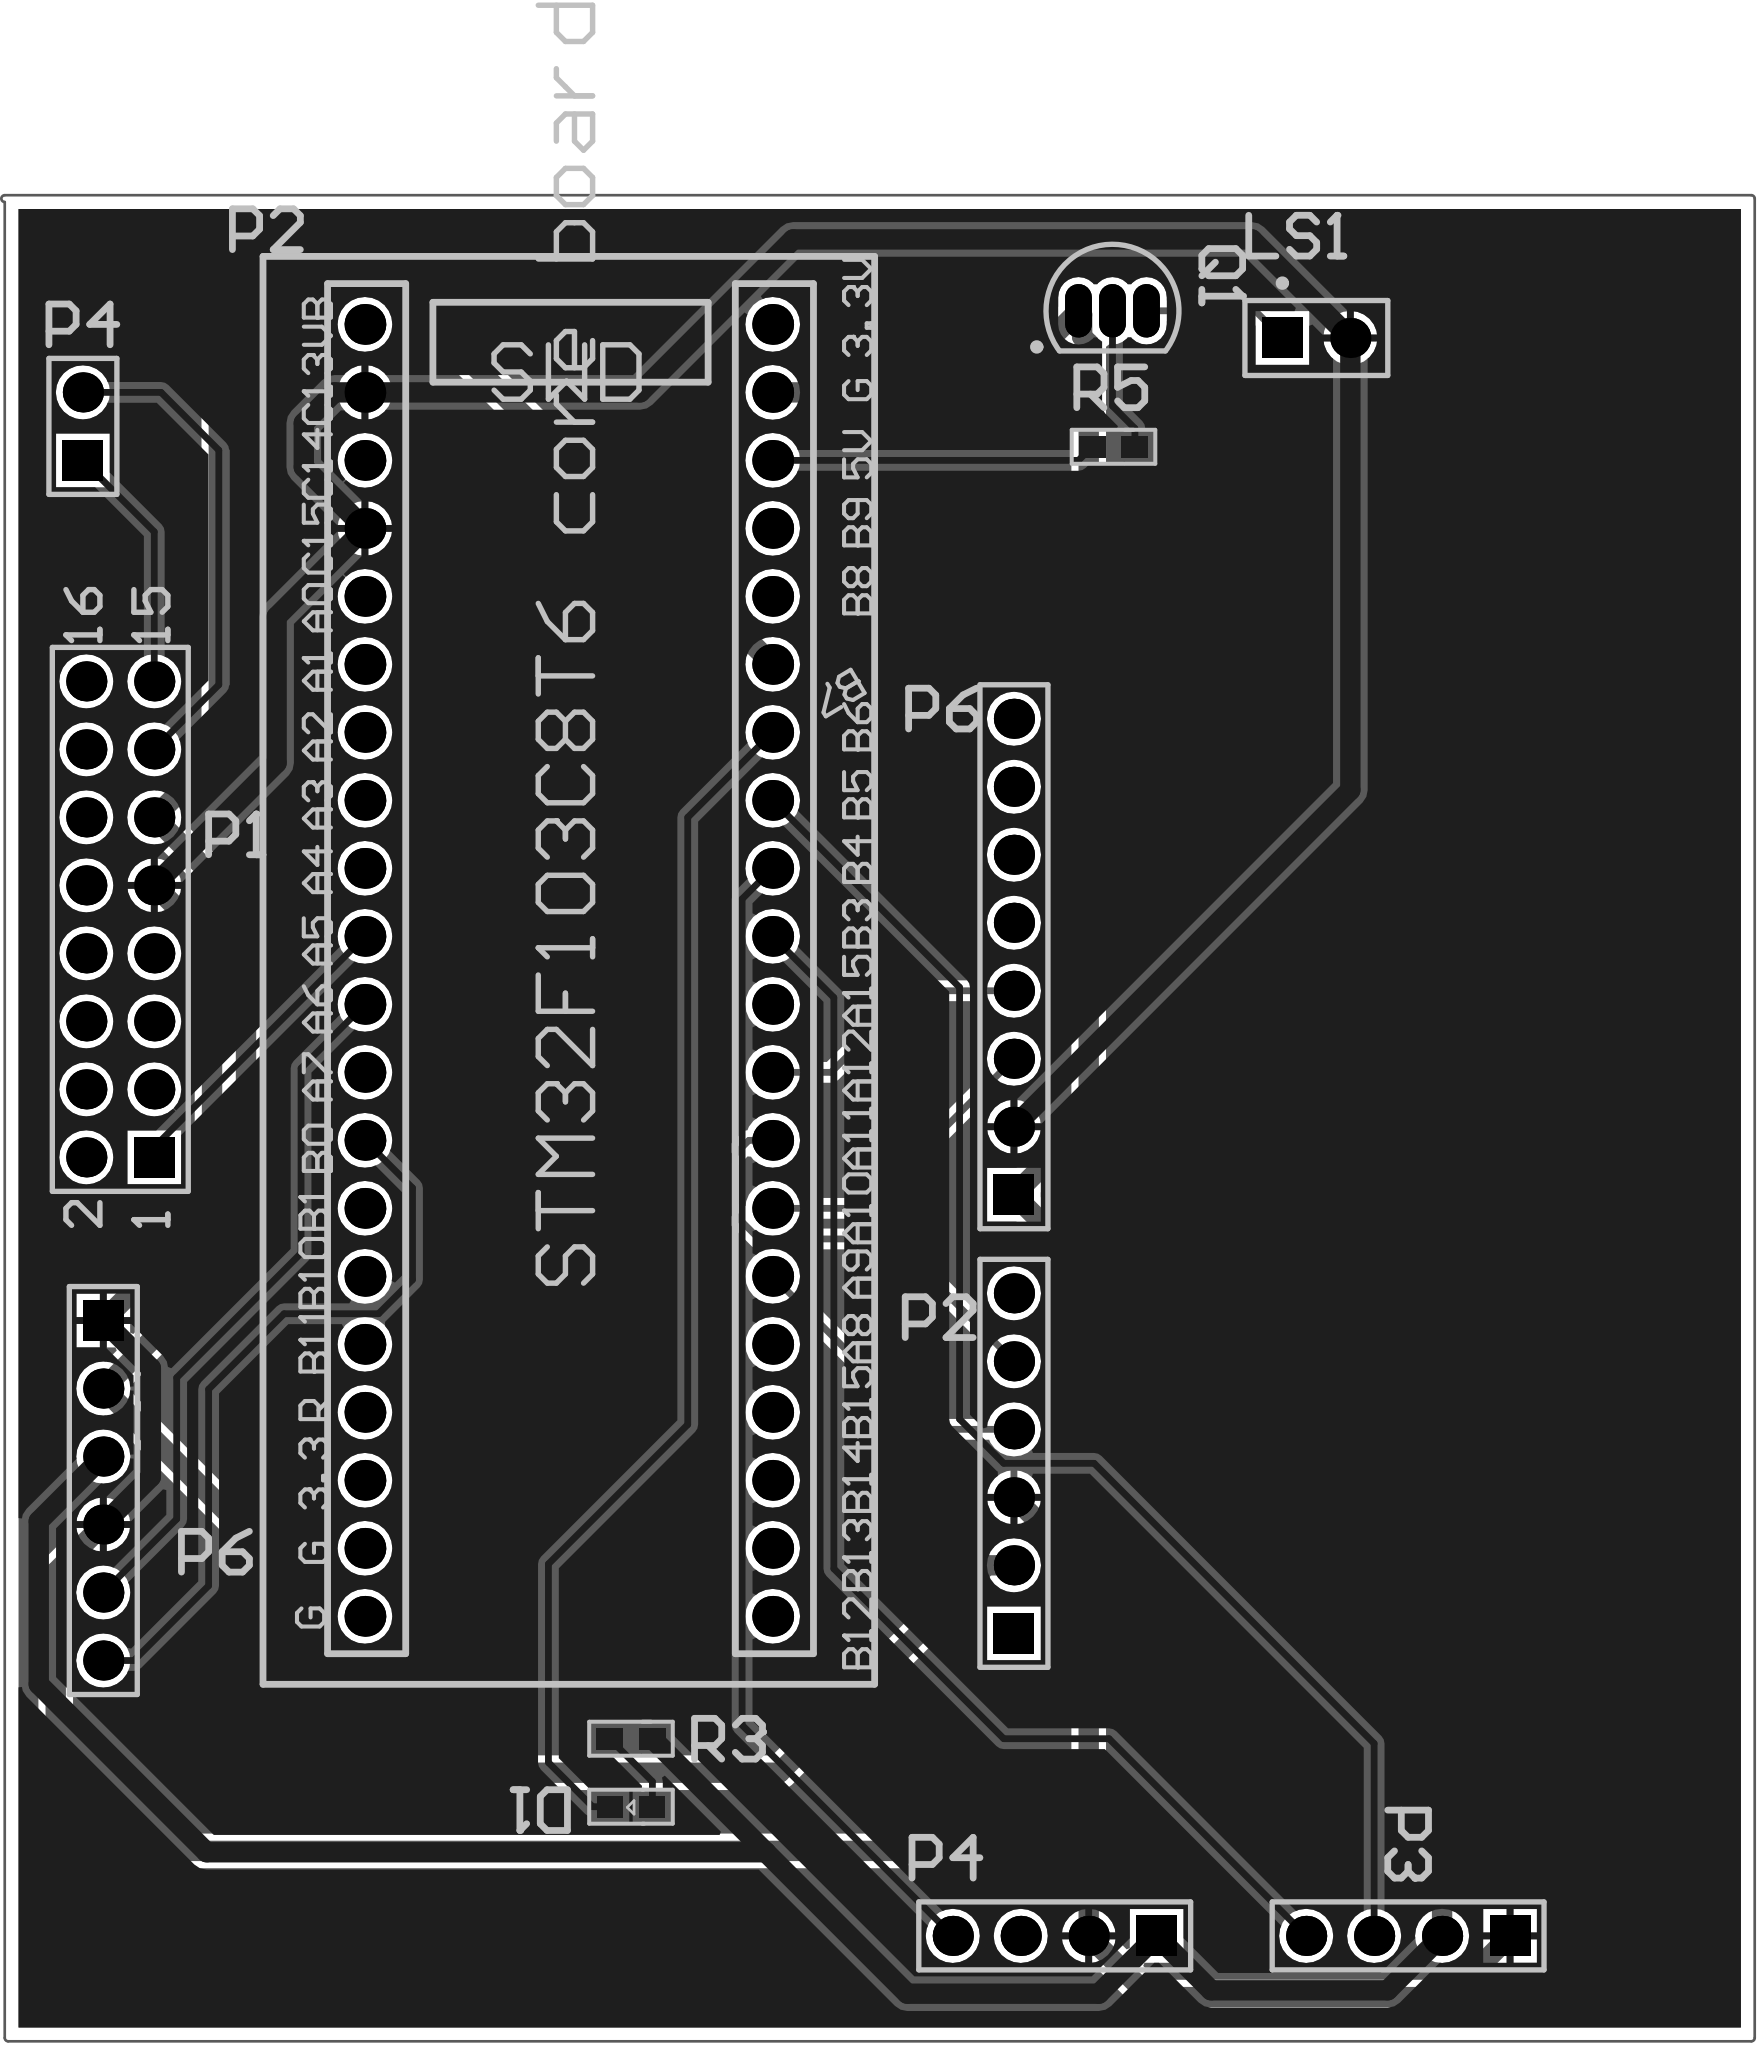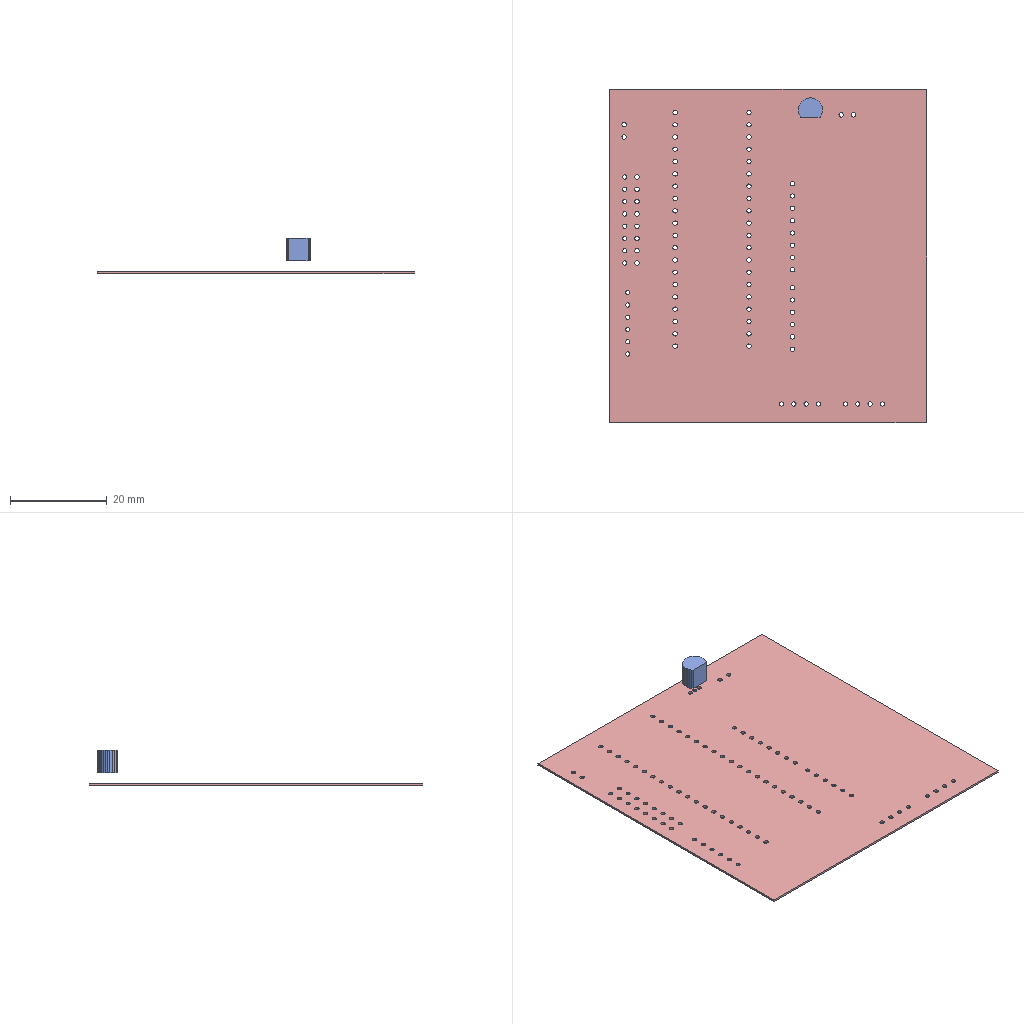Circuit board layout | Altium Designer | box 65.5 x 69 x 7.3 mm
Layer stack:
# Altium Designer layer stack of  (unit mm; dielectric type: 0 none, 1 core, 2 prepreg, 3 surface material)
index,name,kind,layer,copper_thickness_mm,dielectric_type,dielectric_thickness_mm,dielectric_material,dielectric_constant
0,Top Paste,other,,,,,,
1,Top Overlay,other,,,,,,
2,Top Solder,dielectric,,,3,0.0102,Solder Resist,3.5
3,Top Layer,copper,Top Layer,0.0356,,,,
4,Dielectric 1,dielectric,,,0,0.32,FR-4,4.8
5,Bottom Layer,copper,Bottom Layer,0.0356,,,,
6,Bottom Solder,dielectric,,,3,0.0102,Solder Resist,3.5
7,Bottom Overlay,other,,,,,,
8,Bottom Paste,other,,,,,,
# drill layer pairs: low layer,high layer
drill_pair,Top Layer,Bottom Layer
Part placement:
Designator,Comment,Layer,Footprint,Center-X(mm),Center-Y(mm),Rotation
D1,LED0,TopLayer,my0603LED,105.956,28.194,180
LS1,beef,TopLayer,PIN2,131.572,83.058,0
P1,JQ8900,TopLayer,HDR2X8,86.868,61.341,90
P2,JDY-31,TopLayer,HDR1X6,120.269,41.021,90
P2,STM32F103,TopLayer,STM32核心板,103.632,59.436,0
P3,0.96oled,TopLayer,HDR1X4,135.001,23.368,180
P4,Photoresistor,TopLayer,HDR1X4,121.793,23.368,180
P4,Speaker,TopLayer,HDR1X2,85.471,79.756,90
P6,MPU-6050,TopLayer,HDR1X8,120.269,59.944,90
P6,SIM900A,TopLayer,HDR1X6,86.233,40.005,270
Q1,8550,TopLayer,TO-92A,123.952,84.074,270
R3,510R,TopLayer,my0603,105.956,30.734,360
R5,1k,TopLayer,my0603,123.99,78.994,360
Pad and via stacks:
# Altium Designer via and pad stacks of  (unit mm). Each distinct definition once, with the count of objects using it.
# via: kind,start_layer,end_layer,hole_mm,diameter_mm,mode(0 simple;1 top-mid-bottom;2 full stack),diameter_per_layer,count,example_net
# pad: kind,layer,hole_mm,hole_type(0 round;1 square;2 slot),plating,top_size,top_shape(1 round;2 rect;3 octagon;9 rounded rect),mid_size,bottom_size,mode,footprint,size_per_layer,count,example
pad,Top Layer,0,0,plated,1x0.8,2,1x0.8,1x0.8,0,my0603,,4,R3.2
pad,Top Layer,0,0,plated,0.965x0.8,2,0.965x0.8,0.965x0.8,0,my0603LED,,2,D1.1
pad,Multi-Layer,0.9,0,plated,1.5x1.5,1,1.5x1.5,1.5x1.5,0,HDR1X6,,10,P2.6
pad,Multi-Layer,0.9,0,plated,1.5x1.5,2,1.5x1.5,1.5x1.5,0,HDR1X6,,2,P2.1
pad,Multi-Layer,0.9,0,plated,1.5x1.5,1,1.5x1.5,1.5x1.5,0,HDR1X2,,1,P4.2
pad,Multi-Layer,0.9,0,plated,1.5x1.5,2,1.5x1.5,1.5x1.5,0,HDR1X2,,1,P4.1
pad,Multi-Layer,0.9,0,plated,1.5x1.5,1,1.5x1.5,1.5x1.5,0,HDR2X8,,15,P1.16
pad,Multi-Layer,0.9,0,plated,1.5x1.5,2,1.5x1.5,1.5x1.5,0,HDR2X8,,1,P1.1
pad,Multi-Layer,0.9,0,plated,1.5x1.5,2,1.5x1.5,1.5x1.5,0,HDR1X4,,2,P3.1
pad,Multi-Layer,0.9,0,plated,1.5x1.5,1,1.5x1.5,1.5x1.5,0,HDR1X4,,6,P3.2
pad,Multi-Layer,0.9144,2,plated,1.524x1.524,1,1.524x1.524,1.524x1.524,0,STM32\u00BA\u00CB\u00D0\u00C4\u00B0\u00E5,,40,P2.40
pad,Multi-Layer,0.9,0,plated,1.5x1.5,1,1.5x1.5,1.5x1.5,0,PIN2,,1,LS1.2
pad,Multi-Layer,0.9,0,plated,1.5x1.5,2,1.5x1.5,1.5x1.5,0,PIN2,,1,LS1.1
pad,Multi-Layer,0.9,0,plated,2x1,1,2x1,2x1,0,TO-92A,,3,Q1.1
pad,Multi-Layer,0.9,0,plated,1.5x1.5,1,1.5x1.5,1.5x1.5,0,HDR1X8,,7,P6.8
pad,Multi-Layer,0.9,0,plated,1.5x1.5,2,1.5x1.5,1.5x1.5,0,HDR1X8,,1,P6.1
Copper pours:
name,layer,net,type(0 solid;1 hatched;2 none)
Top Layer-No Net,Top Layer,GND,0
Top Layer-No Net,Bottom Layer,GND,0
Design rules, without the lines most boards share:
# Altium Designer design rules of  (exported by Altium Designer, unit mm)
# columns: name | kind | enabled | priority | scope1 | scope2 | descriptor | typed fields (field=value)
Clearance | 0 | enabled | 1 | All | All | Clearance Constraint (Gap=10mil) (All),(All) | gap=0.254
PlaneConnect | 6 | enabled | 1 | All | All | Power Plane Connect Rule(Relief Connect )(Expansion=20mil) (Conductor Width=10mil) (Air Gap=10mil) (Entries=4) (All) | relief_conductor_width=0.254 relief_entries=4 relief_expansion=0.508
PolygonConnect | 20 | enabled | 1 | All | All | Polygon Connect Rule(Relief Connect )(Conductor Width=10mil) (Relief Angle=90 Angle) (Entries=4) (Air Gap Width=10mil) (All),(All) | connect_style(0=relief,1=direct,2=none)=0 relief_conductor_width=0.254 relief_entries=4
Width | 2 | enabled | 1 | All | All | Width Constraint (Min=10mil) (Max=30mil) (Preferred=10mil) (All) |
RoutingVias | 11 | enabled | 1 | All | All | Routing Via (MinHoleWidth=28mil) (MaxHoleWidth=28mil) (PreferredHoleWidth=28mil) (MinWidth=50mil) (MaxWidth=50mil) (PreferedWidth=50mil) (All) | via_min_hole=0.7112 via_max_hole=0.7112 via_preferred_diameter=1.27 via_preferred_hole=0.7112
PasteMaskExpansion | 14 | enabled | 1 | All | All | Paste Mask Expansion (Expansion =0mil) (All) | expansion=0
SolderMaskExpansion | 13 | enabled | 1 | All | All | Solder Mask Expansion (Expansion =4mil) (All) | expansion=0.1016
DiffPairsRouting | 51 | enabled | 1 | All | All | Differential Pairs Uncoupled Length using the Gap Constraints (Min=10mil) (Max=10mil) (Prefered=10mil)  and Width Constraints (Min=15mil) (Max=15mil) (Prefered=15mil) (All) |
HoleToHoleClearance | 52 | enabled | 1 | All | All | Hole To Hole Clearance (Gap=10mil) (All),(All) | gap=0.254
MinimumSolderMaskSliver | 53 | enabled | 1 | All | All | Minimum Solder Mask Sliver (Gap=0mil) (All),(All) |
SilkToSolderMaskClearance | 54 | enabled | 1 | IsPad | All | Silk To Solder Mask (Clearance=0mil) (IsPad),(All) |
SilkToSilkClearance | 55 | enabled | 1 | All | All | Silk to Silk (Clearance=0mil) (All),(All) |